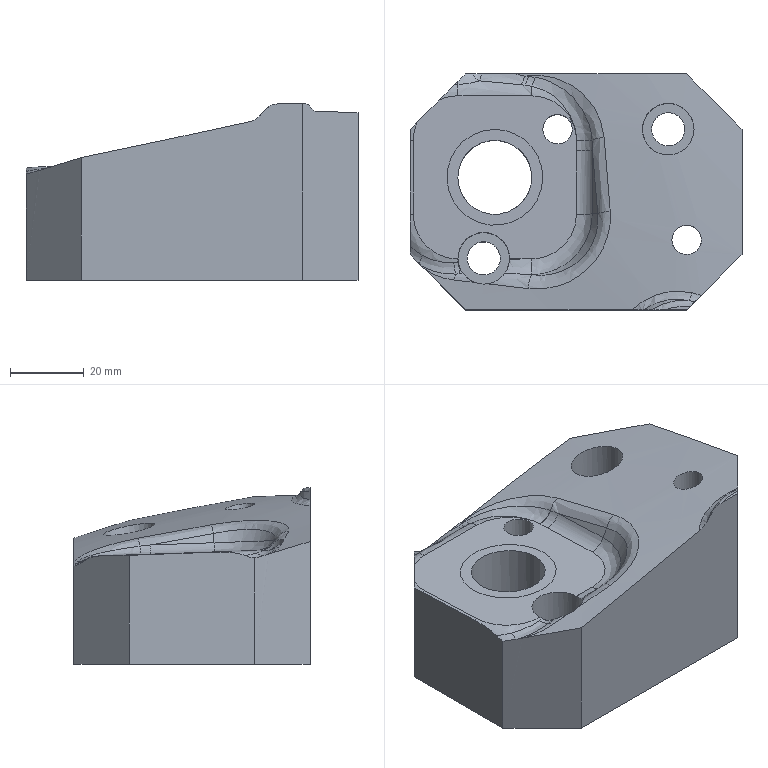Part | NX | features solid 2 | 1 solid | 61 faces | box 90 x 64.003 x 47.871 mm | volume 162899 mm3 | spline 43 | plane 11 | cylinder 7 | commonest cylinder face diameters 8 x2 9 x2 14 x2 20.05 x1